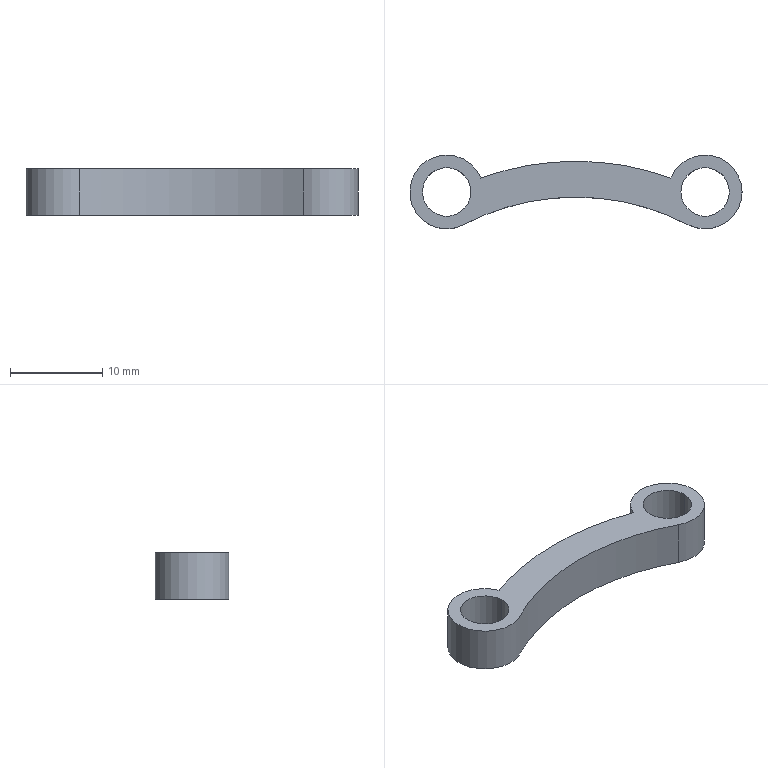Part | SolidWorks | features ICE 5, Attribute 1, Extrusion 1 | 1 solid | 11 faces | box 36 x 8 x 5 mm | volume 695.737 mm3 | cylinder 9 | plane 2 | commonest cylinder face diameters 5.25 x4 8 x3 52.473 x1 60.244 x1
STEP:
#1=CARTESIAN_POINT('',(-30.625,0.,0.));
#2=VERTEX_POINT('',#1);
#3=CARTESIAN_POINT('',(-25.375,0.,0.));
#4=VERTEX_POINT('',#3);
#5=CARTESIAN_POINT('',(-28.,0.,0.));
#6=DIRECTION('',(0.,0.,1.));
#7=DIRECTION('',(1.,0.,0.));
#8=AXIS2_PLACEMENT_3D('',#5,#6,#7);
#9=CIRCLE('',#8,2.625);
#10=EDGE_CURVE('',#2,#4,#9,.T.);
#11=ORIENTED_EDGE('',*,*,#10,.F.);
#12=CARTESIAN_POINT('',(-30.625,0.,5.));
#13=VERTEX_POINT('',#12);
#14=CARTESIAN_POINT('',(-30.625,0.,0.));
#15=DIRECTION('',(0.,0.,1.));
#16=VECTOR('',#15,1000.);
#17=LINE('',#14,#16);
#18=EDGE_CURVE('',#2,#13,#17,.T.);
#19=ORIENTED_EDGE('',*,*,#18,.T.);
#20=CARTESIAN_POINT('',(-25.375,0.,5.));
#21=VERTEX_POINT('',#20);
#22=CARTESIAN_POINT('',(-28.,0.,5.));
#23=DIRECTION('',(0.,0.,1.));
#24=DIRECTION('',(1.,0.,0.));
#25=AXIS2_PLACEMENT_3D('',#22,#23,#24);
#26=CIRCLE('',#25,2.625);
#27=EDGE_CURVE('',#13,#21,#26,.T.);
#28=ORIENTED_EDGE('',*,*,#27,.T.);
#29=CARTESIAN_POINT('',(-25.375,0.,0.));
#30=DIRECTION('',(0.,0.,1.));
#31=VECTOR('',#30,1000.);
#32=LINE('',#29,#31);
#33=EDGE_CURVE('',#4,#21,#32,.T.);
#34=ORIENTED_EDGE('',*,*,#33,.F.);
#35=EDGE_LOOP('',(#11,#19,#28,#34));
#36=FACE_OUTER_BOUND('',#35,.T.);
#37=CARTESIAN_POINT('',(-28.,0.,0.));
#38=DIRECTION('',(0.,0.,1.));
#39=DIRECTION('',(1.,0.,0.));
#40=AXIS2_PLACEMENT_3D('',#37,#38,#39);
#41=CYLINDRICAL_SURFACE('',#40,2.625);
#42=ADVANCED_FACE('',(#36),#41,.F.);
#43=CARTESIAN_POINT('',(-2.625,0.,0.));
#44=VERTEX_POINT('',#43);
#45=CARTESIAN_POINT('',(2.625,0.,0.));
#46=VERTEX_POINT('',#45);
#47=CARTESIAN_POINT('',(0.,0.,0.));
#48=DIRECTION('',(0.,0.,1.));
#49=DIRECTION('',(1.,0.,0.));
#50=AXIS2_PLACEMENT_3D('',#47,#48,#49);
#51=CIRCLE('',#50,2.625);
#52=EDGE_CURVE('',#44,#46,#51,.T.);
#53=ORIENTED_EDGE('',*,*,#52,.F.);
#54=CARTESIAN_POINT('',(-2.625,0.,5.));
#55=VERTEX_POINT('',#54);
#56=CARTESIAN_POINT('',(-2.625,0.,0.));
#57=DIRECTION('',(0.,0.,1.));
#58=VECTOR('',#57,1000.);
#59=LINE('',#56,#58);
#60=EDGE_CURVE('',#44,#55,#59,.T.);
#61=ORIENTED_EDGE('',*,*,#60,.T.);
#62=CARTESIAN_POINT('',(2.625,0.,5.));
#63=VERTEX_POINT('',#62);
#64=CARTESIAN_POINT('',(0.,0.,5.));
#65=DIRECTION('',(0.,0.,1.));
#66=DIRECTION('',(1.,0.,0.));
#67=AXIS2_PLACEMENT_3D('',#64,#65,#66);
#68=CIRCLE('',#67,2.625);
#69=EDGE_CURVE('',#55,#63,#68,.T.);
#70=ORIENTED_EDGE('',*,*,#69,.T.);
#71=CARTESIAN_POINT('',(2.625,0.,0.));
#72=DIRECTION('',(0.,0.,1.));
#73=VECTOR('',#72,1000.);
#74=LINE('',#71,#73);
#75=EDGE_CURVE('',#46,#63,#74,.T.);
#76=ORIENTED_EDGE('',*,*,#75,.F.);
#77=EDGE_LOOP('',(#53,#61,#70,#76));
#78=FACE_OUTER_BOUND('',#77,.T.);
#79=CARTESIAN_POINT('',(0.,0.,0.));
#80=DIRECTION('',(0.,0.,1.));
#81=DIRECTION('',(1.,0.,0.));
#82=AXIS2_PLACEMENT_3D('',#79,#80,#81);
#83=CYLINDRICAL_SURFACE('',#82,2.625);
#84=ADVANCED_FACE('',(#78),#83,.F.);
#85=CARTESIAN_POINT('',(-1.852,-3.545,0.));
#86=VERTEX_POINT('',#85);
#87=CARTESIAN_POINT('',(4.,0.,0.));
#88=VERTEX_POINT('',#87);
#89=CARTESIAN_POINT('',(0.,0.,0.));
#90=DIRECTION('',(0.,0.,1.));
#91=DIRECTION('',(1.,0.,0.));
#92=AXIS2_PLACEMENT_3D('',#89,#90,#91);
#93=CIRCLE('',#92,4.);
#94=EDGE_CURVE('',#86,#88,#93,.T.);
#95=ORIENTED_EDGE('',*,*,#94,.T.);
#96=CARTESIAN_POINT('',(4.,0.,5.));
#97=VERTEX_POINT('',#96);
#98=CARTESIAN_POINT('',(4.,0.,0.));
#99=DIRECTION('',(0.,0.,1.));
#100=VECTOR('',#99,1000.);
#101=LINE('',#98,#100);
#102=EDGE_CURVE('',#88,#97,#101,.T.);
#103=ORIENTED_EDGE('',*,*,#102,.T.);
#104=CARTESIAN_POINT('',(-1.852,-3.545,5.));
#105=VERTEX_POINT('',#104);
#106=CARTESIAN_POINT('',(0.,0.,5.));
#107=DIRECTION('',(0.,0.,1.));
#108=DIRECTION('',(1.,0.,0.));
#109=AXIS2_PLACEMENT_3D('',#106,#107,#108);
#110=CIRCLE('',#109,4.);
#111=EDGE_CURVE('',#105,#97,#110,.T.);
#112=ORIENTED_EDGE('',*,*,#111,.F.);
#113=CARTESIAN_POINT('',(-1.852,-3.545,0.));
#114=DIRECTION('',(0.,0.,1.));
#115=VECTOR('',#114,1000.);
#116=LINE('',#113,#115);
#117=EDGE_CURVE('',#86,#105,#116,.T.);
#118=ORIENTED_EDGE('',*,*,#117,.F.);
#119=EDGE_LOOP('',(#95,#103,#112,#118));
#120=FACE_OUTER_BOUND('',#119,.T.);
#121=CARTESIAN_POINT('',(0.,0.,0.));
#122=DIRECTION('',(0.,0.,1.));
#123=DIRECTION('',(1.,0.,0.));
#124=AXIS2_PLACEMENT_3D('',#121,#122,#123);
#125=CYLINDRICAL_SURFACE('',#124,4.);
#126=ADVANCED_FACE('',(#120),#125,.T.);
#127=CARTESIAN_POINT('',(0.,0.,5.));
#128=DIRECTION('',(0.,0.,1.));
#129=DIRECTION('',(1.,0.,0.));
#130=AXIS2_PLACEMENT_3D('',#127,#128,#129);
#131=CIRCLE('',#130,2.625);
#132=EDGE_CURVE('',#63,#55,#131,.T.);
#133=ORIENTED_EDGE('',*,*,#132,.F.);
#134=ORIENTED_EDGE('',*,*,#69,.F.);
#135=EDGE_LOOP('',(#133,#134));
#136=FACE_BOUND('',#135,.T.);
#137=CARTESIAN_POINT('',(-28.,0.,5.));
#138=DIRECTION('',(0.,0.,1.));
#139=DIRECTION('',(1.,0.,0.));
#140=AXIS2_PLACEMENT_3D('',#137,#138,#139);
#141=CIRCLE('',#140,2.625);
#142=EDGE_CURVE('',#21,#13,#141,.T.);
#143=ORIENTED_EDGE('',*,*,#142,.F.);
#144=ORIENTED_EDGE('',*,*,#27,.F.);
#145=EDGE_LOOP('',(#143,#144));
#146=FACE_BOUND('',#145,.T.);
#147=CARTESIAN_POINT('',(-24.295,1.508,5.));
#148=VERTEX_POINT('',#147);
#149=CARTESIAN_POINT('',(-26.148,-3.545,5.));
#150=VERTEX_POINT('',#149);
#151=CARTESIAN_POINT('',(-28.,0.,5.));
#152=DIRECTION('',(0.,0.,1.));
#153=DIRECTION('',(1.,0.,0.));
#154=AXIS2_PLACEMENT_3D('',#151,#152,#153);
#155=CIRCLE('',#154,4.);
#156=EDGE_CURVE('',#148,#150,#155,.T.);
#157=ORIENTED_EDGE('',*,*,#156,.T.);
#158=CARTESIAN_POINT('',(-14.,-26.8,5.));
#159=DIRECTION('',(0.,0.,-1.));
#160=DIRECTION('',(-1.,0.,0.));
#161=AXIS2_PLACEMENT_3D('',#158,#159,#160);
#162=CIRCLE('',#161,26.236);
#163=EDGE_CURVE('',#150,#105,#162,.T.);
#164=ORIENTED_EDGE('',*,*,#163,.T.);
#165=ORIENTED_EDGE('',*,*,#111,.T.);
#166=CARTESIAN_POINT('',(-3.705,1.508,5.));
#167=VERTEX_POINT('',#166);
#168=CARTESIAN_POINT('',(0.,0.,5.));
#169=DIRECTION('',(0.,0.,1.));
#170=DIRECTION('',(1.,0.,0.));
#171=AXIS2_PLACEMENT_3D('',#168,#169,#170);
#172=CIRCLE('',#171,4.);
#173=EDGE_CURVE('',#97,#167,#172,.T.);
#174=ORIENTED_EDGE('',*,*,#173,.T.);
#175=CARTESIAN_POINT('',(-14.,-26.8,5.));
#176=DIRECTION('',(0.,0.,-1.));
#177=DIRECTION('',(1.,0.,0.));
#178=AXIS2_PLACEMENT_3D('',#175,#176,#177);
#179=CIRCLE('',#178,30.122);
#180=EDGE_CURVE('',#148,#167,#179,.T.);
#181=ORIENTED_EDGE('',*,*,#180,.F.);
#182=EDGE_LOOP('',(#157,#164,#165,#174,#181));
#183=FACE_OUTER_BOUND('',#182,.T.);
#184=CARTESIAN_POINT('',(-7.,-11.9,5.));
#185=DIRECTION('',(0.,0.,-1.));
#186=DIRECTION('',(-1.,0.,0.));
#187=AXIS2_PLACEMENT_3D('',#184,#185,#186);
#188=PLANE('',#187);
#189=ADVANCED_FACE('',(#136,#146,#183),#188,.F.);
#190=CARTESIAN_POINT('',(-26.148,-3.545,0.));
#191=VERTEX_POINT('',#190);
#192=CARTESIAN_POINT('',(-14.,-26.8,0.));
#193=DIRECTION('',(0.,0.,-1.));
#194=DIRECTION('',(-1.,0.,0.));
#195=AXIS2_PLACEMENT_3D('',#192,#193,#194);
#196=CIRCLE('',#195,26.236);
#197=EDGE_CURVE('',#191,#86,#196,.T.);
#198=ORIENTED_EDGE('',*,*,#197,.F.);
#199=CARTESIAN_POINT('',(-24.295,1.508,0.));
#200=VERTEX_POINT('',#199);
#201=CARTESIAN_POINT('',(-28.,0.,0.));
#202=DIRECTION('',(0.,0.,1.));
#203=DIRECTION('',(1.,0.,0.));
#204=AXIS2_PLACEMENT_3D('',#201,#202,#203);
#205=CIRCLE('',#204,4.);
#206=EDGE_CURVE('',#200,#191,#205,.T.);
#207=ORIENTED_EDGE('',*,*,#206,.F.);
#208=CARTESIAN_POINT('',(-3.705,1.508,0.));
#209=VERTEX_POINT('',#208);
#210=CARTESIAN_POINT('',(-14.,-26.8,0.));
#211=DIRECTION('',(0.,0.,-1.));
#212=DIRECTION('',(1.,0.,0.));
#213=AXIS2_PLACEMENT_3D('',#210,#211,#212);
#214=CIRCLE('',#213,30.122);
#215=EDGE_CURVE('',#200,#209,#214,.T.);
#216=ORIENTED_EDGE('',*,*,#215,.T.);
#217=CARTESIAN_POINT('',(0.,0.,0.));
#218=DIRECTION('',(0.,0.,1.));
#219=DIRECTION('',(1.,0.,0.));
#220=AXIS2_PLACEMENT_3D('',#217,#218,#219);
#221=CIRCLE('',#220,4.);
#222=EDGE_CURVE('',#88,#209,#221,.T.);
#223=ORIENTED_EDGE('',*,*,#222,.F.);
#224=ORIENTED_EDGE('',*,*,#94,.F.);
#225=EDGE_LOOP('',(#198,#207,#216,#223,#224));
#226=FACE_OUTER_BOUND('',#225,.T.);
#227=CARTESIAN_POINT('',(-28.,0.,0.));
#228=DIRECTION('',(0.,0.,1.));
#229=DIRECTION('',(1.,0.,0.));
#230=AXIS2_PLACEMENT_3D('',#227,#228,#229);
#231=CIRCLE('',#230,2.625);
#232=EDGE_CURVE('',#4,#2,#231,.T.);
#233=ORIENTED_EDGE('',*,*,#232,.T.);
#234=ORIENTED_EDGE('',*,*,#10,.T.);
#235=EDGE_LOOP('',(#233,#234));
#236=FACE_BOUND('',#235,.T.);
#237=CARTESIAN_POINT('',(0.,0.,0.));
#238=DIRECTION('',(0.,0.,1.));
#239=DIRECTION('',(1.,0.,0.));
#240=AXIS2_PLACEMENT_3D('',#237,#238,#239);
#241=CIRCLE('',#240,2.625);
#242=EDGE_CURVE('',#46,#44,#241,.T.);
#243=ORIENTED_EDGE('',*,*,#242,.T.);
#244=ORIENTED_EDGE('',*,*,#52,.T.);
#245=EDGE_LOOP('',(#243,#244));
#246=FACE_BOUND('',#245,.T.);
#247=CARTESIAN_POINT('',(-7.,-11.9,0.));
#248=DIRECTION('',(0.,0.,-1.));
#249=DIRECTION('',(-1.,0.,0.));
#250=AXIS2_PLACEMENT_3D('',#247,#248,#249);
#251=PLANE('',#250);
#252=ADVANCED_FACE('',(#226,#236,#246),#251,.T.);
#253=CARTESIAN_POINT('',(-26.148,-3.545,0.));
#254=DIRECTION('',(0.,0.,1.));
#255=VECTOR('',#254,1000.);
#256=LINE('',#253,#255);
#257=EDGE_CURVE('',#191,#150,#256,.T.);
#258=ORIENTED_EDGE('',*,*,#257,.T.);
#259=ORIENTED_EDGE('',*,*,#156,.F.);
#260=CARTESIAN_POINT('',(-24.295,1.508,0.));
#261=DIRECTION('',(0.,0.,1.));
#262=VECTOR('',#261,1000.);
#263=LINE('',#260,#262);
#264=EDGE_CURVE('',#200,#148,#263,.T.);
#265=ORIENTED_EDGE('',*,*,#264,.F.);
#266=ORIENTED_EDGE('',*,*,#206,.T.);
#267=EDGE_LOOP('',(#258,#259,#265,#266));
#268=FACE_OUTER_BOUND('',#267,.T.);
#269=CARTESIAN_POINT('',(-28.,0.,0.));
#270=DIRECTION('',(0.,0.,1.));
#271=DIRECTION('',(1.,0.,0.));
#272=AXIS2_PLACEMENT_3D('',#269,#270,#271);
#273=CYLINDRICAL_SURFACE('',#272,4.);
#274=ADVANCED_FACE('',(#268),#273,.T.);
#275=ORIENTED_EDGE('',*,*,#102,.F.);
#276=ORIENTED_EDGE('',*,*,#222,.T.);
#277=CARTESIAN_POINT('',(-3.705,1.508,0.));
#278=DIRECTION('',(0.,0.,1.));
#279=VECTOR('',#278,1000.);
#280=LINE('',#277,#279);
#281=EDGE_CURVE('',#209,#167,#280,.T.);
#282=ORIENTED_EDGE('',*,*,#281,.T.);
#283=ORIENTED_EDGE('',*,*,#173,.F.);
#284=EDGE_LOOP('',(#275,#276,#282,#283));
#285=FACE_OUTER_BOUND('',#284,.T.);
#286=CARTESIAN_POINT('',(0.,0.,0.));
#287=DIRECTION('',(0.,0.,1.));
#288=DIRECTION('',(1.,0.,0.));
#289=AXIS2_PLACEMENT_3D('',#286,#287,#288);
#290=CYLINDRICAL_SURFACE('',#289,4.);
#291=ADVANCED_FACE('',(#285),#290,.T.);
#292=ORIENTED_EDGE('',*,*,#60,.F.);
#293=ORIENTED_EDGE('',*,*,#242,.F.);
#294=ORIENTED_EDGE('',*,*,#75,.T.);
#295=ORIENTED_EDGE('',*,*,#132,.T.);
#296=EDGE_LOOP('',(#292,#293,#294,#295));
#297=FACE_OUTER_BOUND('',#296,.T.);
#298=CARTESIAN_POINT('',(0.,0.,0.));
#299=DIRECTION('',(0.,0.,1.));
#300=DIRECTION('',(1.,0.,0.));
#301=AXIS2_PLACEMENT_3D('',#298,#299,#300);
#302=CYLINDRICAL_SURFACE('',#301,2.625);
#303=ADVANCED_FACE('',(#297),#302,.F.);
#304=ORIENTED_EDGE('',*,*,#18,.F.);
#305=ORIENTED_EDGE('',*,*,#232,.F.);
#306=ORIENTED_EDGE('',*,*,#33,.T.);
#307=ORIENTED_EDGE('',*,*,#142,.T.);
#308=EDGE_LOOP('',(#304,#305,#306,#307));
#309=FACE_OUTER_BOUND('',#308,.T.);
#310=CARTESIAN_POINT('',(-28.,0.,0.));
#311=DIRECTION('',(0.,0.,1.));
#312=DIRECTION('',(1.,0.,0.));
#313=AXIS2_PLACEMENT_3D('',#310,#311,#312);
#314=CYLINDRICAL_SURFACE('',#313,2.625);
#315=ADVANCED_FACE('',(#309),#314,.F.);
#316=ORIENTED_EDGE('',*,*,#180,.T.);
#317=ORIENTED_EDGE('',*,*,#281,.F.);
#318=ORIENTED_EDGE('',*,*,#215,.F.);
#319=ORIENTED_EDGE('',*,*,#264,.T.);
#320=EDGE_LOOP('',(#316,#317,#318,#319));
#321=FACE_OUTER_BOUND('',#320,.T.);
#322=CARTESIAN_POINT('',(-14.,-26.8,0.));
#323=DIRECTION('',(0.,0.,1.));
#324=DIRECTION('',(1.,0.,0.));
#325=AXIS2_PLACEMENT_3D('',#322,#323,#324);
#326=CYLINDRICAL_SURFACE('',#325,30.122);
#327=ADVANCED_FACE('',(#321),#326,.T.);
#328=ORIENTED_EDGE('',*,*,#163,.F.);
#329=ORIENTED_EDGE('',*,*,#257,.F.);
#330=ORIENTED_EDGE('',*,*,#197,.T.);
#331=ORIENTED_EDGE('',*,*,#117,.T.);
#332=EDGE_LOOP('',(#328,#329,#330,#331));
#333=FACE_OUTER_BOUND('',#332,.T.);
#334=CARTESIAN_POINT('',(-14.,-26.8,0.));
#335=DIRECTION('',(0.,0.,1.));
#336=DIRECTION('',(1.,0.,0.));
#337=AXIS2_PLACEMENT_3D('',#334,#335,#336);
#338=CYLINDRICAL_SURFACE('',#337,26.236);
#339=ADVANCED_FACE('',(#333),#338,.F.);
#340=CLOSED_SHELL('',(#42,#84,#126,#189,#252,#274,#291,#303,#315,#327,#339));
#341=MANIFOLD_SOLID_BREP('',#340);
#342=CARTESIAN_POINT('',(0.,0.,0.));
#343=DIRECTION('',(0.,0.,1.));
#344=DIRECTION('',(1.,0.,0.));
#345=AXIS2_PLACEMENT_3D('',#342,#343,#344);
#346=(LENGTH_UNIT()NAMED_UNIT(*)SI_UNIT(.MILLI.,.METRE.));
#347=UNCERTAINTY_MEASURE_WITH_UNIT(LENGTH_MEASURE(0.00001),#346,'','');
#348=(NAMED_UNIT(*)PLANE_ANGLE_UNIT()SI_UNIT($,.RADIAN.));
#349=(NAMED_UNIT(*)SI_UNIT($,.STERADIAN.)SOLID_ANGLE_UNIT());
#350=(GEOMETRIC_REPRESENTATION_CONTEXT(3)GLOBAL_UNCERTAINTY_ASSIGNED_CONTEXT((#347))GLOBAL_UNIT_ASSIGNED_CONTEXT((#346,#348,#349))REPRESENTATION_CONTEXT('',''));
#351=ADVANCED_BREP_SHAPE_REPRESENTATION('',(#341,#345),#350);